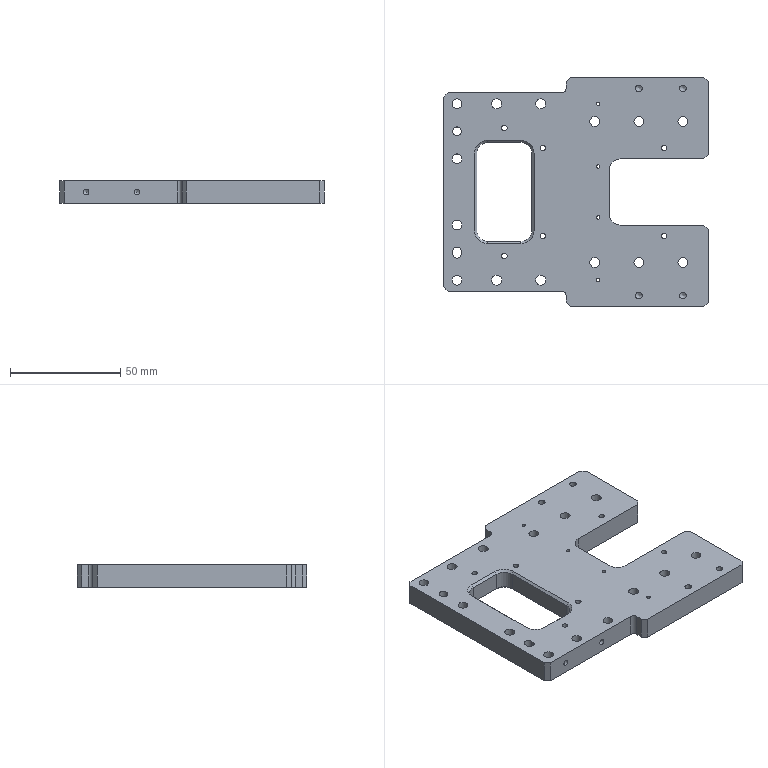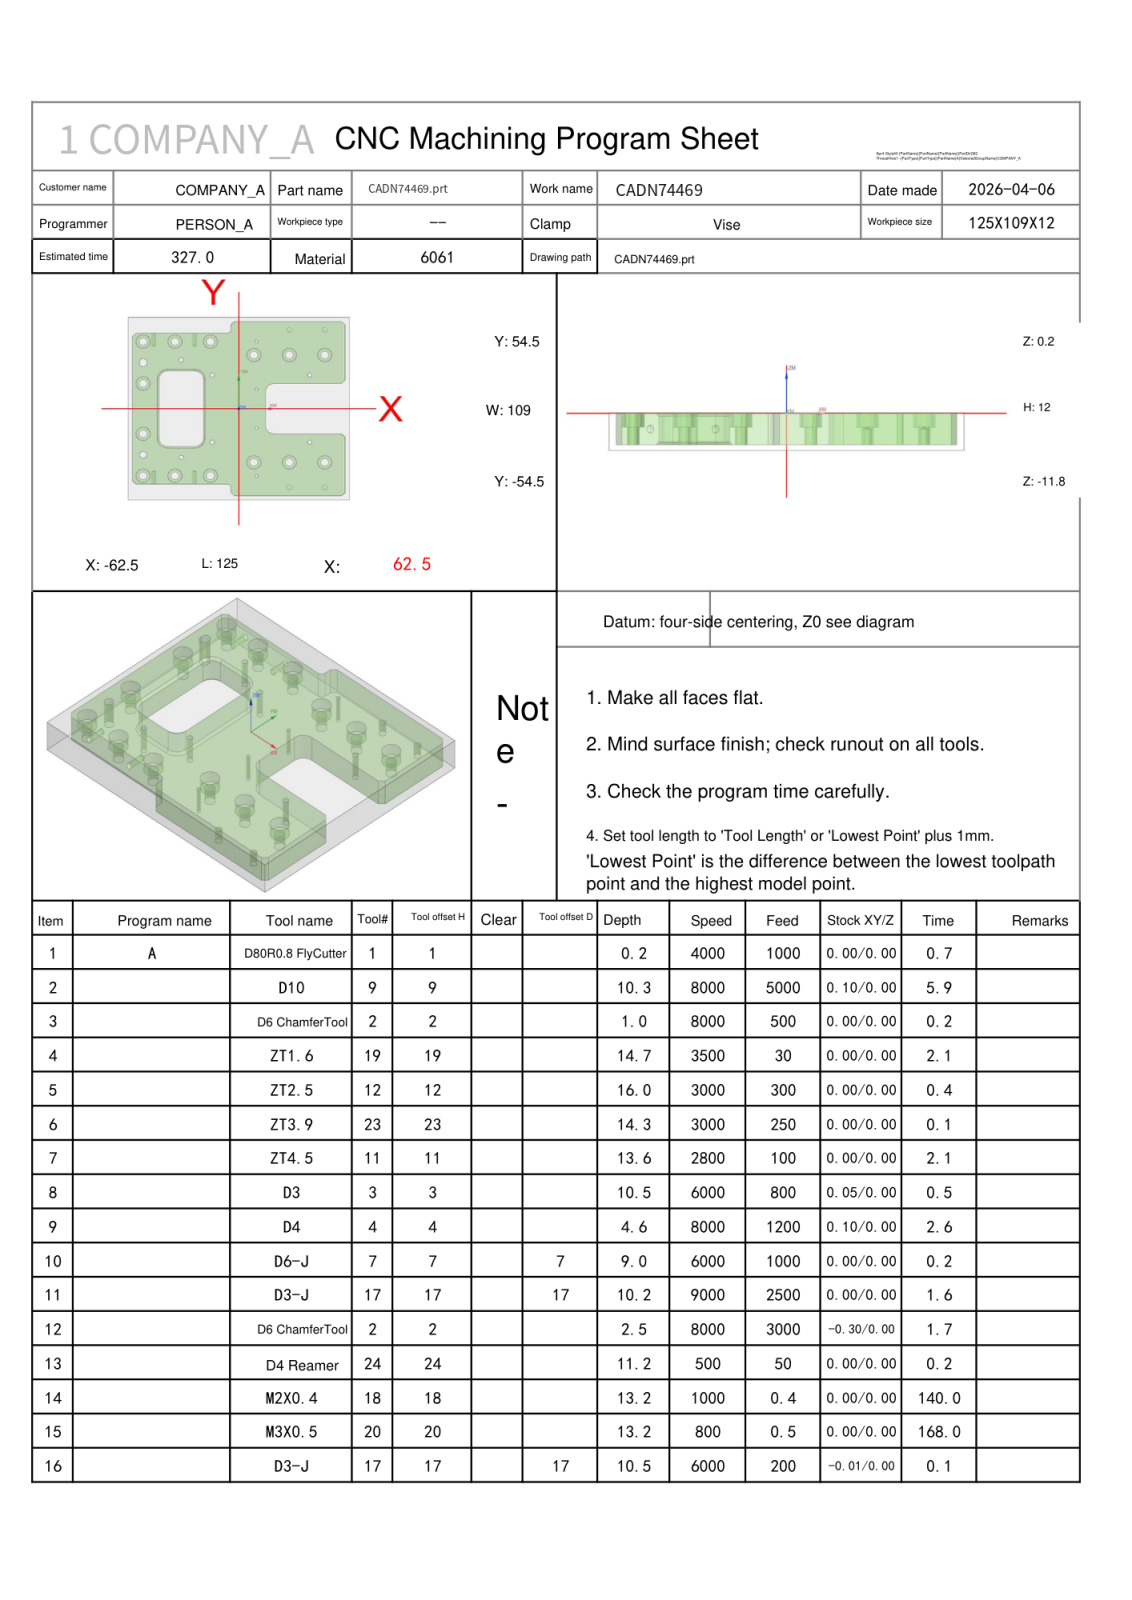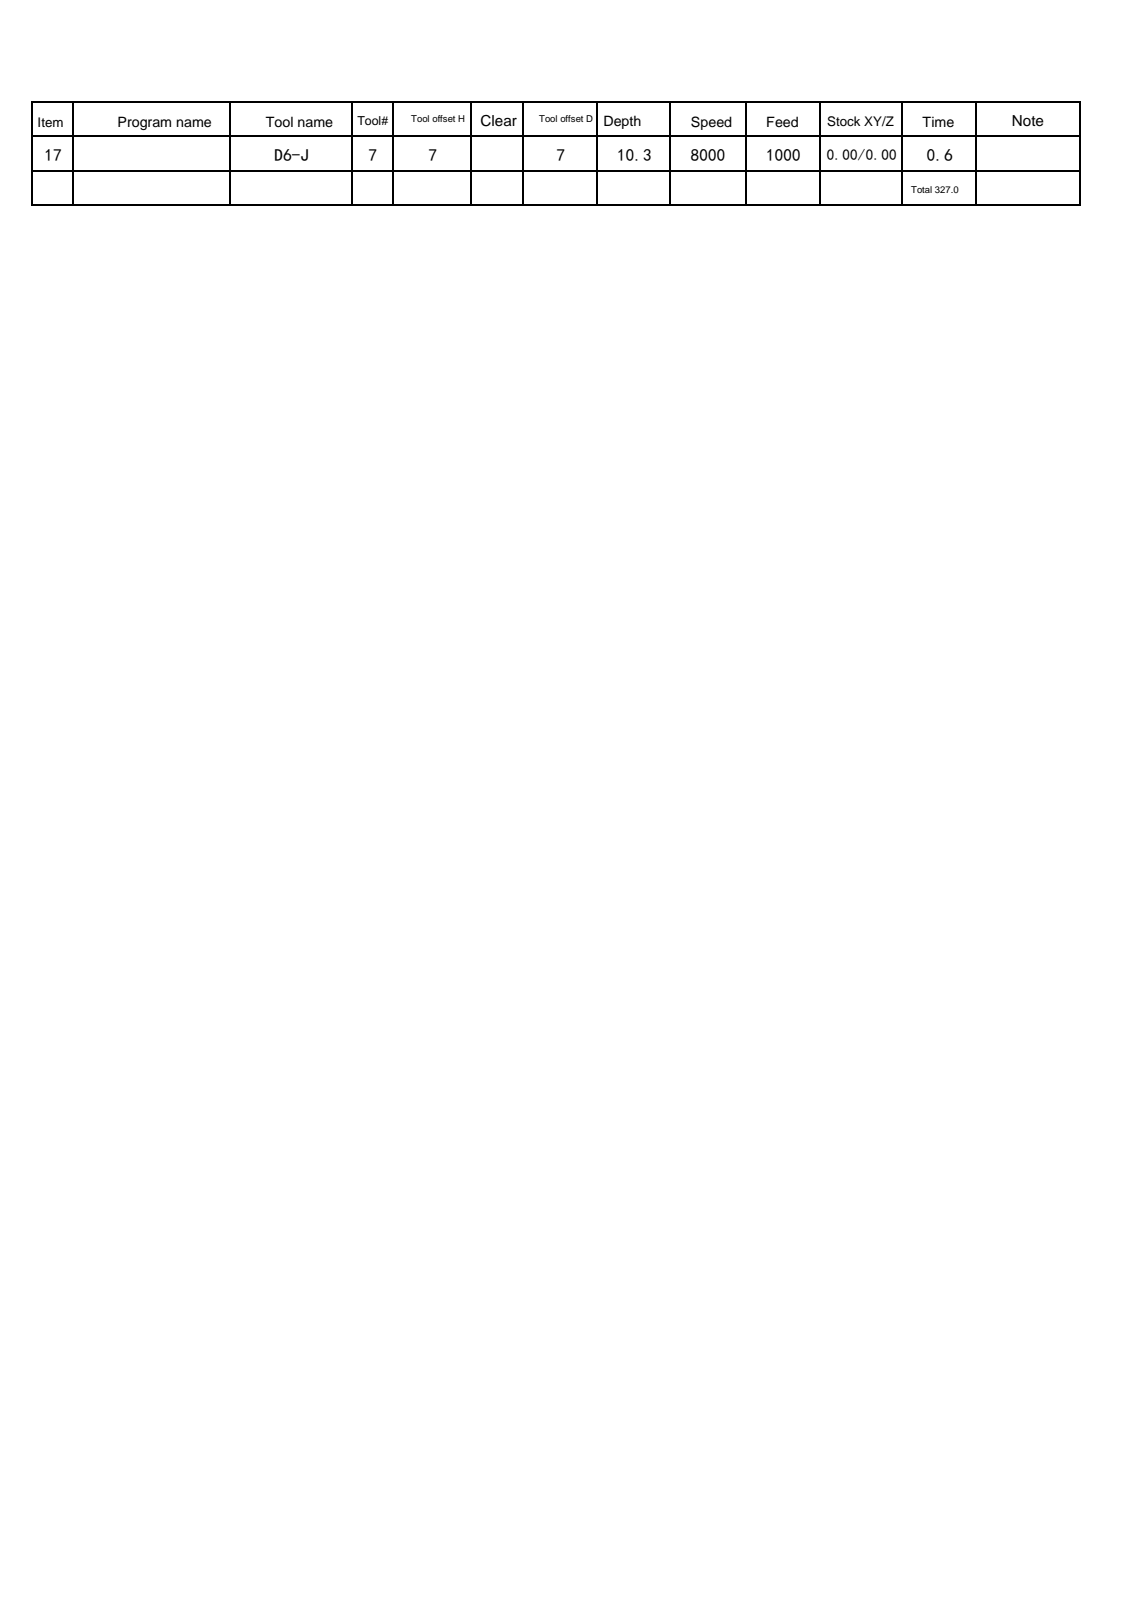NC program | NX | posted by the shop | part box 120 x 104 x 10 mm
Lines 2469 to 3517 of 6435:
N3 T02 M06
(D6 ChamferTool  D=6. R=0. H=02 ce=0.00 di=0.00)
G00 G90 G54 X48.5 Y-32. M03 S8000
G43 H02 Z20.
M08
G98 G81 X48.5 Y-32. Z-.8 R1. F500.
X40. Y-20.
X28.5 Y-32.
X10. Y-40.
X8.5 Y-32.
X10. Y-11.54
Y11.54
X40. Y20.
X48.5 Y32.
X28.5
X10. Y40.
X8.5 Y32.
X-16. Y40.
X-15. Y20.
X-32.5 Y29.
X-36. Y40.
X-54.
Y15.
Y-15.
Y-27.5
Y-40.
X-36.
X-32.5 Y-29.
X-15. Y-20.
X-16. Y-40.
X-54. Y27.
G80
G00 Z20.
G91 G28 Z0.0
M05
M09
G91 G28 Z0.0
M01
N4 T19 M06
(ZT1.6 D=1.6 DR_a=118 H=19)
G00 G90 G54 X10. Y40. M03 S3500
G43 H19 Z20.
M08
G98 G83 X10. Y40. Z-14.481 R1. F30. Q1.
Y11.54
Y-11.54
Y-40.
G80
G00 Z20.
G91 G28 Z0.0
M05
M09
G91 G28 Z0.0
M01
N5 T12 M06
(ZT2.5 D=2.5 DR_a=118 H=12)
G00 G90 G54 X40. Y20. M03 S3000
G43 H12 Z20.
M08
G98 G83 X40. Y20. Z-15.751 R1. F300. Q2.
Y-20.
X-15.
X-32.5 Y-29.
X-15. Y20.
X-32.5 Y29.
G80
G00 Z20.
G91 G28 Z0.0
M05
M09
G91 G28 Z0.0
M01
N6 T23 M06
(ZT3.9 D=3.9 DR_a=120 H=23)
G00 G90 G54 X-54. Y-27.5 M03 S3000
G43 H23 Z20.
M08
G98 G83 X-54. Y-27.5 Z-14.126 R1. F250. Q2.
Y27.
G80
G00 Z20.
G91 G28 Z0.0
M05
M09
G91 G28 Z0.0
M01
N7 T11 M06
(ZT4.5 D=4.5 DR_a=118 H=11)
G00 G90 G54 X48.5 Y-32. M03 S2800
G43 H11 Z20.
M08
G98 G83 X48.5 Y-32. Z-13.352 R1. F100. Q2.
X28.5
X8.5
X-16. Y-40.
X-36.
X-54.
Y-15.
Y15.
Y40.
X-36.
X-16.
X8.5 Y32.
X28.5
X48.5
G80
G00 Z20.
G91 G28 Z0.0
M05
M09
G91 G28 Z0.0
M01
N8 T03 M06
(D3  D=3. R=0. H=03 ce=0.05 di=0.00)
G00 G90 G54 X-54.45 Y27.5 M03 S6000
G43 H03 Z20.
M08
Z.5
G01 Y27. Z.485 F800.
G03 X-54. Y26.55 Z.463 I.45 J0.0
X-53.55 Y27. Z.441 I0.0 J.45
G01 Y28. Z.411
G03 X-54. Y28.45 Z.389 I-.45 J0.0
X-54.45 Y28. Z.367 I0.0 J-.45
G01 Y27. Z.337
G03 X-54. Y26.55 Z.315 I.45 J0.0
X-53.55 Y27. Z.293 I0.0 J.45
G01 Y28. Z.263
G03 X-54. Y28.45 Z.241 I-.45 J0.0
X-54.45 Y28. Z.219 I0.0 J-.45
G01 Y27. Z.189
G03 X-54. Y26.55 Z.167 I.45 J0.0
X-53.55 Y27. Z.145 I0.0 J.45
G01 Y28. Z.115
G03 X-54. Y28.45 Z.093 I-.45 J0.0
X-54.45 Y28. Z.071 I0.0 J-.45
G01 Y27. Z.041
G03 X-54. Y26.55 Z.019 I.45 J0.0
X-53.55 Y27. Z-.002 I0.0 J.45
G01 Y28. Z-.033
G03 X-54. Y28.45 Z-.055 I-.45 J0.0
X-54.45 Y28. Z-.076 I0.0 J-.45
G01 Y27. Z-.107
G03 X-54. Y26.55 Z-.129 I.45 J0.0
X-53.55 Y27. Z-.15 I0.0 J.45
G01 Y28. Z-.181
G03 X-54. Y28.45 Z-.203 I-.45 J0.0
X-54.45 Y28. Z-.224 I0.0 J-.45
G01 Y27. Z-.255
G03 X-54. Y26.55 Z-.277 I.45 J0.0
X-53.55 Y27. Z-.298 I0.0 J.45
G01 Y28. Z-.329
G03 X-54. Y28.45 Z-.351 I-.45 J0.0
X-54.45 Y28. Z-.372 I0.0 J-.45
G01 Y27. Z-.403
G03 X-54. Y26.55 Z-.425 I.45 J0.0
X-53.55 Y27. Z-.446 I0.0 J.45
G01 Y28. Z-.477
G03 X-54. Y28.45 Z-.499 I-.45 J0.0
X-54.45 Y28. Z-.52 I0.0 J-.45
G01 Y27. Z-.551
G03 X-54. Y26.55 Z-.573 I.45 J0.0
X-53.55 Y27. Z-.594 I0.0 J.45
G01 Y28. Z-.625
G03 X-54. Y28.45 Z-.647 I-.45 J0.0
X-54.45 Y28. Z-.668 I0.0 J-.45
G01 Y27. Z-.699
G03 X-54. Y26.55 Z-.721 I.45 J0.0
X-53.55 Y27. Z-.742 I0.0 J.45
G01 Y28. Z-.773
G03 X-54. Y28.45 Z-.795 I-.45 J0.0
X-54.45 Y28. Z-.816 I0.0 J-.45
G01 Y27. Z-.847
G03 X-54. Y26.55 Z-.868 I.45 J0.0
X-53.55 Y27. Z-.89 I0.0 J.45
G01 Y28. Z-.921
G03 X-54. Y28.45 Z-.942 I-.45 J0.0
X-54.45 Y28. Z-.964 I0.0 J-.45
G01 Y27. Z-.995
G03 X-54. Y26.55 Z-1.016 I.45 J0.0
X-53.55 Y27. Z-1.038 I0.0 J.45
G01 Y28. Z-1.069
G03 X-54. Y28.45 Z-1.09 I-.45 J0.0
X-54.45 Y28. Z-1.112 I0.0 J-.45
G01 Y27. Z-1.143
G03 X-54. Y26.55 Z-1.164 I.45 J0.0
X-53.55 Y27. Z-1.186 I0.0 J.45
G01 Y28. Z-1.217
G03 X-54. Y28.45 Z-1.238 I-.45 J0.0
X-54.45 Y28. Z-1.26 I0.0 J-.45
G01 Y27. Z-1.291
G03 X-54. Y26.55 Z-1.312 I.45 J0.0
X-53.55 Y27. Z-1.334 I0.0 J.45
G01 Y28. Z-1.365
G03 X-54. Y28.45 Z-1.386 I-.45 J0.0
X-54.45 Y28. Z-1.408 I0.0 J-.45
G01 Y27. Z-1.439
G03 X-54. Y26.55 Z-1.46 I.45 J0.0
X-53.55 Y27. Z-1.482 I0.0 J.45
G01 Y28. Z-1.513
G03 X-54. Y28.45 Z-1.534 I-.45 J0.0
X-54.45 Y28. Z-1.556 I0.0 J-.45
G01 Y27. Z-1.587
G03 X-54. Y26.55 Z-1.608 I.45 J0.0
X-53.55 Y27. Z-1.63 I0.0 J.45
G01 Y28. Z-1.661
G03 X-54. Y28.45 Z-1.682 I-.45 J0.0
X-54.45 Y28. Z-1.704 I0.0 J-.45
G01 Y27. Z-1.735
G03 X-54. Y26.55 Z-1.756 I.45 J0.0
X-53.55 Y27. Z-1.778 I0.0 J.45
G01 Y28. Z-1.808
G03 X-54. Y28.45 Z-1.83 I-.45 J0.0
X-54.45 Y28. Z-1.852 I0.0 J-.45
G01 Y27. Z-1.882
G03 X-54. Y26.55 Z-1.904 I.45 J0.0
X-53.55 Y27. Z-1.926 I0.0 J.45
G01 Y28. Z-1.956
G03 X-54. Y28.45 Z-1.978 I-.45 J0.0
X-54.45 Y28. Z-2. I0.0 J-.45
G01 Y27. Z-2.03
G03 X-54. Y26.55 Z-2.052 I.45 J0.0
X-53.55 Y27. Z-2.074 I0.0 J.45
G01 Y28. Z-2.104
G03 X-54. Y28.45 Z-2.126 I-.45 J0.0
X-54.45 Y28. Z-2.148 I0.0 J-.45
G01 Y27. Z-2.178
G03 X-54. Y26.55 Z-2.2 I.45 J0.0
X-53.55 Y27. Z-2.222 I0.0 J.45
G01 Y28. Z-2.252
G03 X-54. Y28.45 Z-2.274 I-.45 J0.0
X-54.45 Y28. Z-2.296 I0.0 J-.45
G01 Y27. Z-2.326
G03 X-54. Y26.55 Z-2.348 I.45 J0.0
X-53.55 Y27. Z-2.37 I0.0 J.45
G01 Y28. Z-2.4
G03 X-54. Y28.45 Z-2.422 I-.45 J0.0
X-54.45 Y28. Z-2.444 I0.0 J-.45
G01 Y27. Z-2.474
G03 X-54. Y26.55 Z-2.496 I.45 J0.0
X-53.55 Y27. Z-2.518 I0.0 J.45
G01 Y28. Z-2.548
G03 X-54. Y28.45 Z-2.57 I-.45 J0.0
X-54.45 Y28. Z-2.592 I0.0 J-.45
G01 Y27. Z-2.622
G03 X-54. Y26.55 Z-2.644 I.45 J0.0
X-53.55 Y27. Z-2.665 I0.0 J.45
G01 Y28. Z-2.696
G03 X-54. Y28.45 Z-2.718 I-.45 J0.0
X-54.45 Y28. Z-2.739 I0.0 J-.45
G01 Y27. Z-2.77
G03 X-54. Y26.55 Z-2.792 I.45 J0.0
X-53.55 Y27. Z-2.813 I0.0 J.45
G01 Y28. Z-2.844
G03 X-54. Y28.45 Z-2.866 I-.45 J0.0
X-54.45 Y28. Z-2.887 I0.0 J-.45
G01 Y27. Z-2.918
G03 X-54. Y26.55 Z-2.94 I.45 J0.0
X-53.55 Y27. Z-2.961 I0.0 J.45
G01 Y28. Z-2.992
G03 X-54. Y28.45 Z-3.014 I-.45 J0.0
X-54.45 Y28. Z-3.035 I0.0 J-.45
G01 Y27. Z-3.066
G03 X-54. Y26.55 Z-3.088 I.45 J0.0
X-53.55 Y27. Z-3.109 I0.0 J.45
G01 Y28. Z-3.14
G03 X-54. Y28.45 Z-3.162 I-.45 J0.0
X-54.45 Y28. Z-3.183 I0.0 J-.45
G01 Y27. Z-3.214
G03 X-54. Y26.55 Z-3.236 I.45 J0.0
X-53.55 Y27. Z-3.257 I0.0 J.45
G01 Y28. Z-3.288
G03 X-54. Y28.45 Z-3.31 I-.45 J0.0
X-54.45 Y28. Z-3.331 I0.0 J-.45
G01 Y27. Z-3.362
G03 X-54. Y26.55 Z-3.384 I.45 J0.0
X-53.55 Y27. Z-3.405 I0.0 J.45
G01 Y28. Z-3.436
G03 X-54. Y28.45 Z-3.458 I-.45 J0.0
X-54.45 Y28. Z-3.479 I0.0 J-.45
G01 Y27. Z-3.51
G03 X-54. Y26.55 Z-3.532 I.45 J0.0
X-53.55 Y27. Z-3.553 I0.0 J.45
G01 Y28. Z-3.584
G03 X-54. Y28.45 Z-3.605 I-.45 J0.0
X-54.45 Y28. Z-3.627 I0.0 J-.45
G01 Y27. Z-3.658
G03 X-54. Y26.55 Z-3.679 I.45 J0.0
X-53.55 Y27. Z-3.701 I0.0 J.45
G01 Y28. Z-3.732
G03 X-54. Y28.45 Z-3.753 I-.45 J0.0
X-54.45 Y28. Z-3.775 I0.0 J-.45
G01 Y27. Z-3.806
G03 X-54. Y26.55 Z-3.827 I.45 J0.0
X-53.55 Y27. Z-3.849 I0.0 J.45
G01 Y28. Z-3.88
G03 X-54. Y28.45 Z-3.901 I-.45 J0.0
X-54.45 Y28. Z-3.923 I0.0 J-.45
G01 Y27. Z-3.954
G03 X-54. Y26.55 Z-3.975 I.45 J0.0
X-53.55 Y27. Z-3.997 I0.0 J.45
G01 Y28. Z-4.028
G03 X-54. Y28.45 Z-4.049 I-.45 J0.0
X-54.45 Y28. Z-4.071 I0.0 J-.45
G01 Y27. Z-4.102
G03 X-54. Y26.55 Z-4.123 I.45 J0.0
X-53.55 Y27. Z-4.145 I0.0 J.45
G01 Y28. Z-4.176
G03 X-54. Y28.45 Z-4.197 I-.45 J0.0
X-54.45 Y28. Z-4.219 I0.0 J-.45
G01 Y27. Z-4.25
G03 X-54. Y26.55 Z-4.271 I.45 J0.0
X-53.55 Y27. Z-4.293 I0.0 J.45
G01 Y28. Z-4.324
G03 X-54. Y28.45 Z-4.345 I-.45 J0.0
X-54.45 Y28. Z-4.367 I0.0 J-.45
G01 Y27. Z-4.398
G03 X-54. Y26.55 Z-4.419 I.45 J0.0
X-53.55 Y27. Z-4.441 I0.0 J.45
G01 Y28. Z-4.471
G03 X-54. Y28.45 Z-4.493 I-.45 J0.0
X-54.45 Y28. Z-4.515 I0.0 J-.45
G01 Y27. Z-4.545
G03 X-54. Y26.55 Z-4.567 I.45 J0.0
X-53.55 Y27. Z-4.589 I0.0 J.45
G01 Y28. Z-4.619
G03 X-54. Y28.45 Z-4.641 I-.45 J0.0
X-54.45 Y28. Z-4.663 I0.0 J-.45
G01 Y27. Z-4.693
G03 X-54. Y26.55 Z-4.715 I.45 J0.0
X-53.55 Y27. Z-4.737 I0.0 J.45
G01 Y28. Z-4.767
G03 X-54. Y28.45 Z-4.789 I-.45 J0.0
X-54.45 Y28. Z-4.811 I0.0 J-.45
G01 Y27. Z-4.841
G03 X-54. Y26.55 Z-4.863 I.45 J0.0
X-53.55 Y27. Z-4.885 I0.0 J.45
G01 Y28. Z-4.915
G03 X-54. Y28.45 Z-4.937 I-.45 J0.0
X-54.45 Y28. Z-4.959 I0.0 J-.45
G01 Y27. Z-4.989
G03 X-54. Y26.55 Z-5.011 I.45 J0.0
X-53.55 Y27. Z-5.033 I0.0 J.45
G01 Y28. Z-5.063
G03 X-54. Y28.45 Z-5.085 I-.45 J0.0
X-54.45 Y28. Z-5.107 I0.0 J-.45
G01 Y27. Z-5.137
G03 X-54. Y26.55 Z-5.159 I.45 J0.0
X-53.55 Y27. Z-5.181 I0.0 J.45
G01 Y28. Z-5.211
G03 X-54. Y28.45 Z-5.233 I-.45 J0.0
X-54.45 Y28. Z-5.255 I0.0 J-.45
G01 Y27. Z-5.285
G03 X-54. Y26.55 Z-5.307 I.45 J0.0
X-53.55 Y27. Z-5.329 I0.0 J.45
G01 Y28. Z-5.359
G03 X-54. Y28.45 Z-5.381 I-.45 J0.0
X-54.45 Y28. Z-5.402 I0.0 J-.45
G01 Y27. Z-5.433
G03 X-54. Y26.55 Z-5.455 I.45 J0.0
X-53.55 Y27. Z-5.476 I0.0 J.45
G01 Y28. Z-5.507
G03 X-54. Y28.45 Z-5.529 I-.45 J0.0
X-54.45 Y28. Z-5.55 I0.0 J-.45
G01 Y27. Z-5.581
G03 X-54. Y26.55 Z-5.603 I.45 J0.0
X-53.55 Y27. Z-5.624 I0.0 J.45
G01 Y28. Z-5.655
G03 X-54. Y28.45 Z-5.677 I-.45 J0.0
X-54.45 Y28. Z-5.698 I0.0 J-.45
G01 Y27. Z-5.729
G03 X-54. Y26.55 Z-5.751 I.45 J0.0
X-53.55 Y27. Z-5.772 I0.0 J.45
G01 Y28. Z-5.803
G03 X-54. Y28.45 Z-5.825 I-.45 J0.0
X-54.45 Y28. Z-5.846 I0.0 J-.45
G01 Y27. Z-5.877
G03 X-54. Y26.55 Z-5.899 I.45 J0.0
X-53.55 Y27. Z-5.92 I0.0 J.45
G01 Y28. Z-5.951
G03 X-54. Y28.45 Z-5.973 I-.45 J0.0
X-54.45 Y28. Z-5.994 I0.0 J-.45
G01 Y27. Z-6.025
G03 X-54. Y26.55 Z-6.047 I.45 J0.0
X-53.55 Y27. Z-6.068 I0.0 J.45
G01 Y28. Z-6.099
G03 X-54. Y28.45 Z-6.121 I-.45 J0.0
X-54.45 Y28. Z-6.142 I0.0 J-.45
G01 Y27. Z-6.173
G03 X-54. Y26.55 Z-6.195 I.45 J0.0
X-53.55 Y27. Z-6.216 I0.0 J.45
G01 Y28. Z-6.247
G03 X-54. Y28.45 Z-6.268 I-.45 J0.0
X-54.45 Y28. Z-6.29 I0.0 J-.45
G01 Y27. Z-6.321
G03 X-54. Y26.55 Z-6.342 I.45 J0.0
X-53.55 Y27. Z-6.364 I0.0 J.45
G01 Y28. Z-6.395
G03 X-54. Y28.45 Z-6.416 I-.45 J0.0
X-54.45 Y28. Z-6.438 I0.0 J-.45
G01 Y27. Z-6.469
G03 X-54. Y26.55 Z-6.49 I.45 J0.0
X-53.55 Y27. Z-6.512 I0.0 J.45
G01 Y28. Z-6.543
G03 X-54. Y28.45 Z-6.564 I-.45 J0.0
X-54.45 Y28. Z-6.586 I0.0 J-.45
G01 Y27. Z-6.617
G03 X-54. Y26.55 Z-6.638 I.45 J0.0
X-53.55 Y27. Z-6.66 I0.0 J.45
G01 Y28. Z-6.691
G03 X-54. Y28.45 Z-6.712 I-.45 J0.0
X-54.45 Y28. Z-6.734 I0.0 J-.45
G01 Y27. Z-6.765
G03 X-54. Y26.55 Z-6.786 I.45 J0.0
X-53.55 Y27. Z-6.808 I0.0 J.45
G01 Y28. Z-6.839
G03 X-54. Y28.45 Z-6.86 I-.45 J0.0
X-54.45 Y28. Z-6.882 I0.0 J-.45
G01 Y27. Z-6.913
G03 X-54. Y26.55 Z-6.934 I.45 J0.0
X-53.55 Y27. Z-6.956 I0.0 J.45
G01 Y28. Z-6.987
G03 X-54. Y28.45 Z-7.008 I-.45 J0.0
X-54.45 Y28. Z-7.03 I0.0 J-.45
G01 Y27. Z-7.061
G03 X-54. Y26.55 Z-7.082 I.45 J0.0
X-53.55 Y27. Z-7.104 I0.0 J.45
G01 Y28. Z-7.135
G03 X-54. Y28.45 Z-7.156 I-.45 J0.0
X-54.45 Y28. Z-7.178 I0.0 J-.45
G01 Y27. Z-7.208
G03 X-54. Y26.55 Z-7.23 I.45 J0.0
X-53.55 Y27. Z-7.252 I0.0 J.45
G01 Y28. Z-7.282
G03 X-54. Y28.45 Z-7.304 I-.45 J0.0
X-54.45 Y28. Z-7.326 I0.0 J-.45
G01 Y27. Z-7.356
G03 X-54. Y26.55 Z-7.378 I.45 J0.0
X-53.55 Y27. Z-7.4 I0.0 J.45
G01 Y28. Z-7.43
G03 X-54. Y28.45 Z-7.452 I-.45 J0.0
X-54.45 Y28. Z-7.474 I0.0 J-.45
G01 Y27. Z-7.504
G03 X-54. Y26.55 Z-7.526 I.45 J0.0
X-53.55 Y27. Z-7.548 I0.0 J.45
G01 Y28. Z-7.578
G03 X-54. Y28.45 Z-7.6 I-.45 J0.0
X-54.45 Y28. Z-7.622 I0.0 J-.45
G01 Y27. Z-7.652
G03 X-54. Y26.55 Z-7.674 I.45 J0.0
X-53.55 Y27. Z-7.696 I0.0 J.45
G01 Y28. Z-7.726
G03 X-54. Y28.45 Z-7.748 I-.45 J0.0
X-54.45 Y28. Z-7.77 I0.0 J-.45
G01 Y27. Z-7.8
G03 X-54. Y26.55 Z-7.822 I.45 J0.0
X-53.55 Y27. Z-7.844 I0.0 J.45
G01 Y28. Z-7.874
G03 X-54. Y28.45 Z-7.896 I-.45 J0.0
X-54.45 Y28. Z-7.918 I0.0 J-.45
G01 Y27. Z-7.948
G03 X-54. Y26.55 Z-7.97 I.45 J0.0
X-53.55 Y27. Z-7.992 I0.0 J.45
G01 Y28. Z-8.022
G03 X-54. Y28.45 Z-8.044 I-.45 J0.0
X-54.45 Y28. Z-8.065 I0.0 J-.45
G01 Y27. Z-8.096
G03 X-54. Y26.55 Z-8.118 I.45 J0.0
X-53.55 Y27. Z-8.139 I0.0 J.45
G01 Y28. Z-8.17
G03 X-54. Y28.45 Z-8.192 I-.45 J0.0
X-54.45 Y28. Z-8.213 I0.0 J-.45
G01 Y27. Z-8.244
G03 X-54. Y26.55 Z-8.266 I.45 J0.0
X-53.55 Y27. Z-8.287 I0.0 J.45
G01 Y28. Z-8.318
G03 X-54. Y28.45 Z-8.34 I-.45 J0.0
X-54.45 Y28. Z-8.361 I0.0 J-.45
G01 Y27. Z-8.392
G03 X-54. Y26.55 Z-8.414 I.45 J0.0
X-53.55 Y27. Z-8.435 I0.0 J.45
G01 Y28. Z-8.466
G03 X-54. Y28.45 Z-8.488 I-.45 J0.0
X-54.45 Y28. Z-8.509 I0.0 J-.45
G01 Y27. Z-8.54
G03 X-54. Y26.55 Z-8.562 I.45 J0.0
X-53.55 Y27. Z-8.583 I0.0 J.45
G01 Y28. Z-8.614
G03 X-54. Y28.45 Z-8.636 I-.45 J0.0
X-54.45 Y28. Z-8.657 I0.0 J-.45
G01 Y27. Z-8.688
G03 X-54. Y26.55 Z-8.71 I.45 J0.0
X-53.55 Y27. Z-8.731 I0.0 J.45
G01 Y28. Z-8.762
G03 X-54. Y28.45 Z-8.784 I-.45 J0.0
X-54.45 Y28. Z-8.805 I0.0 J-.45
G01 Y27. Z-8.836
G03 X-54. Y26.55 Z-8.858 I.45 J0.0
X-53.55 Y27. Z-8.879 I0.0 J.45
G01 Y28. Z-8.91
G03 X-54. Y28.45 Z-8.932 I-.45 J0.0
X-54.45 Y28. Z-8.953 I0.0 J-.45
G01 Y27. Z-8.984
G03 X-54. Y26.55 Z-9.005 I.45 J0.0
X-53.55 Y27. Z-9.027 I0.0 J.45
G01 Y28. Z-9.058
G03 X-54. Y28.45 Z-9.079 I-.45 J0.0
X-54.45 Y28. Z-9.101 I0.0 J-.45
G01 Y27. Z-9.132
G03 X-54. Y26.55 Z-9.153 I.45 J0.0
X-53.55 Y27. Z-9.175 I0.0 J.45
G01 Y28. Z-9.206
G03 X-54. Y28.45 Z-9.227 I-.45 J0.0
X-54.45 Y28. Z-9.249 I0.0 J-.45
G01 Y27. Z-9.28
G03 X-54. Y26.55 Z-9.301 I.45 J0.0
X-53.55 Y27. Z-9.323 I0.0 J.45
G01 Y28. Z-9.354
G03 X-54. Y28.45 Z-9.375 I-.45 J0.0
X-54.45 Y28. Z-9.397 I0.0 J-.45
G01 Y27. Z-9.428
G03 X-54. Y26.55 Z-9.449 I.45 J0.0
X-53.55 Y27. Z-9.471 I0.0 J.45
G01 Y28. Z-9.502
G03 X-54. Y28.45 Z-9.523 I-.45 J0.0
X-54.45 Y28. Z-9.545 I0.0 J-.45
G01 Y27. Z-9.576
G03 X-54. Y26.55 Z-9.597 I.45 J0.0
X-53.55 Y27. Z-9.619 I0.0 J.45
G01 Y28. Z-9.65
G03 X-54. Y28.45 Z-9.671 I-.45 J0.0
X-54.45 Y28. Z-9.693 I0.0 J-.45
G01 Y27. Z-9.724
G03 X-54. Y26.55 Z-9.745 I.45 J0.0
X-53.55 Y27. Z-9.767 I0.0 J.45
G01 Y28. Z-9.798
G03 X-54. Y28.45 Z-9.819 I-.45 J0.0
X-54.45 Y28. Z-9.841 I0.0 J-.45
G01 Y27. Z-9.871
G03 X-54. Y26.55 Z-9.893 I.45 J0.0
X-53.55 Y27. Z-9.915 I0.0 J.45
G01 Y28. Z-9.945
G03 X-54. Y28.45 Z-9.967 I-.45 J0.0
X-54.45 Y28. Z-9.989 I0.0 J-.45
G01 Y27. Z-10.019
G03 X-54. Y26.55 Z-10.041 I.45 J0.0
X-53.55 Y27. Z-10.063 I0.0 J.45
G01 Y28. Z-10.093
G03 X-54. Y28.45 Z-10.115 I-.45 J0.0
X-54.45 Y28. Z-10.137 I0.0 J-.45
G01 Y27. Z-10.167
G03 X-54. Y26.55 Z-10.189 I.45 J0.0
X-53.55 Y27. Z-10.211 I0.0 J.45
G01 Y28. Z-10.241
G03 X-54. Y28.45 Z-10.263 I-.45 J0.0
X-54.45 Y28. Z-10.285 I0.0 J-.45
G01 Y27.5 Z-10.3
Y27.
G03 X-54. Y26.55 I.45 J0.0
X-53.55 Y27. I0.0 J.45
G01 Y28.
G03 X-54. Y28.45 I-.45 J0.0
X-54.45 Y28. I0.0 J-.45
G01 Y27.5
Y27.
Z-9.3
G00 Z20.
G91 G28 Z0.0
M05
M09
G91 G28 Z0.0
M01
N9 T04 M06
(D4  D=4. R=0. H=04 ce=0.10 di=0.00)
G00 G90 G54 X-54. Y15. M03 S8000
G43 H04 Z20.
M08
Z.5
G03 X-53.05 Y14.05 I.95 J0.0 F1200.
X-52.1 Y15. I0.0 J.95
X-52.1 Y15. Z.2 I-1.9 J0.0
X-52.1 Y15. Z-.1 I-1.9 J0.0
X-52.1 Y15. Z-.4 I-1.9 J0.0
X-52.1 Y15. Z-.7 I-1.9 J0.0
X-52.1 Y15. Z-1. I-1.9 J0.0
X-52.1 Y15. Z-1.3 I-1.9 J0.0
X-52.1 Y15. Z-1.6 I-1.9 J0.0
X-52.1 Y15. Z-1.9 I-1.9 J0.0
X-52.1 Y15. Z-2.2 I-1.9 J0.0
X-52.1 Y15. Z-2.5 I-1.9 J0.0
X-52.1 Y15. Z-2.8 I-1.9 J0.0
X-52.1 Y15. Z-3.1 I-1.9 J0.0
X-52.1 Y15. Z-3.4 I-1.9 J0.0
X-52.1 Y15. Z-3.7 I-1.9 J0.0
X-52.1 Y15. Z-4. I-1.9 J0.0
X-52.1 Y15. Z-4.3 I-1.9 J0.0
X-54.95 Y16.645 Z-4.4 I-1.9 J0.0
X-55.9 Y15. I.95 J-1.645
X-54. Y13.1 I1.9 J0.0
X-52.1 Y15. I0.0 J1.9
X-54. Y16.9 I-1.9 J0.0
X-54.95 Y16.645 I0.0 J-1.9
X-55.425 Y15.823 I.475 J-.823
X-54.475 Y14.873 I.95 J0.0
X-54. Y15. I0.0 J.95
G00 Z20.
Y40.
Z.5
G03 X-53.05 Y39.05 I.95 J0.0
X-52.1 Y40. I0.0 J.95
X-52.1 Y40. Z.2 I-1.9 J0.0
X-52.1 Y40. Z-.1 I-1.9 J0.0
X-52.1 Y40. Z-.4 I-1.9 J0.0
X-52.1 Y40. Z-.7 I-1.9 J0.0
X-52.1 Y40. Z-1. I-1.9 J0.0
X-52.1 Y40. Z-1.3 I-1.9 J0.0
X-52.1 Y40. Z-1.6 I-1.9 J0.0
X-52.1 Y40. Z-1.9 I-1.9 J0.0
X-52.1 Y40. Z-2.2 I-1.9 J0.0
X-52.1 Y40. Z-2.5 I-1.9 J0.0
X-52.1 Y40. Z-2.8 I-1.9 J0.0
X-52.1 Y40. Z-3.1 I-1.9 J0.0
X-52.1 Y40. Z-3.4 I-1.9 J0.0
X-52.1 Y40. Z-3.7 I-1.9 J0.0
X-52.1 Y40. Z-4. I-1.9 J0.0
X-52.1 Y40. Z-4.3 I-1.9 J0.0
X-54.95 Y41.645 Z-4.4 I-1.9 J0.0
X-55.9 Y40. I.95 J-1.645
X-54. Y38.1 I1.9 J0.0
X-52.1 Y40. I0.0 J1.9
X-54. Y41.9 I-1.9 J0.0
X-54.95 Y41.645 I0.0 J-1.9
X-55.425 Y40.823 I.475 J-.823
X-54.475 Y39.873 I.95 J0.0
X-54. Y40. I0.0 J.95
G00 Z20.
X-36.
Z.5
G03 X-35.05 Y39.05 I.95 J0.0
X-34.1 Y40. I0.0 J.95
X-34.1 Y40. Z.2 I-1.9 J0.0
X-34.1 Y40. Z-.1 I-1.9 J0.0
X-34.1 Y40. Z-.4 I-1.9 J0.0
X-34.1 Y40. Z-.7 I-1.9 J0.0
X-34.1 Y40. Z-1. I-1.9 J0.0
X-34.1 Y40. Z-1.3 I-1.9 J0.0
X-34.1 Y40. Z-1.6 I-1.9 J0.0
X-34.1 Y40. Z-1.9 I-1.9 J0.0
X-34.1 Y40. Z-2.2 I-1.9 J0.0
X-34.1 Y40. Z-2.5 I-1.9 J0.0
X-34.1 Y40. Z-2.8 I-1.9 J0.0
X-34.1 Y40. Z-3.1 I-1.9 J0.0
X-34.1 Y40. Z-3.4 I-1.9 J0.0
X-34.1 Y40. Z-3.7 I-1.9 J0.0
X-34.1 Y40. Z-4. I-1.9 J0.0
X-34.1 Y40. Z-4.3 I-1.9 J0.0
X-36.95 Y41.645 Z-4.4 I-1.9 J0.0
X-37.9 Y40. I.95 J-1.645
X-36. Y38.1 I1.9 J0.0
X-34.1 Y40. I0.0 J1.9
X-36. Y41.9 I-1.9 J0.0
X-36.95 Y41.645 I0.0 J-1.9
X-37.425 Y40.823 I.475 J-.823
X-36.475 Y39.873 I.95 J0.0
X-36. Y40. I0.0 J.95
G00 Z20.
X-16.
Z.5
G03 X-15.05 Y39.05 I.95 J0.0
X-14.1 Y40. I0.0 J.95
X-14.1 Y40. Z.2 I-1.9 J0.0
X-14.1 Y40. Z-.1 I-1.9 J0.0
X-14.1 Y40. Z-.4 I-1.9 J0.0
X-14.1 Y40. Z-.7 I-1.9 J0.0
X-14.1 Y40. Z-1. I-1.9 J0.0
X-14.1 Y40. Z-1.3 I-1.9 J0.0
X-14.1 Y40. Z-1.6 I-1.9 J0.0
X-14.1 Y40. Z-1.9 I-1.9 J0.0
X-14.1 Y40. Z-2.2 I-1.9 J0.0
X-14.1 Y40. Z-2.5 I-1.9 J0.0
X-14.1 Y40. Z-2.8 I-1.9 J0.0
X-14.1 Y40. Z-3.1 I-1.9 J0.0
X-14.1 Y40. Z-3.4 I-1.9 J0.0
X-14.1 Y40. Z-3.7 I-1.9 J0.0
X-14.1 Y40. Z-4. I-1.9 J0.0
X-14.1 Y40. Z-4.3 I-1.9 J0.0
X-16.95 Y41.645 Z-4.4 I-1.9 J0.0
X-17.9 Y40. I.95 J-1.645
X-16. Y38.1 I1.9 J0.0
X-14.1 Y40. I0.0 J1.9
X-16. Y41.9 I-1.9 J0.0
X-16.95 Y41.645 I0.0 J-1.9
X-17.425 Y40.823 I.475 J-.823
X-16.475 Y39.873 I.95 J0.0
X-16. Y40. I0.0 J.95
G00 Z20.
X8.5 Y32.
Z.5
G03 X9.45 Y31.05 I.95 J0.0
X10.4 Y32. I0.0 J.95
X10.4 Y32. Z.2 I-1.9 J0.0
X10.4 Y32. Z-.1 I-1.9 J0.0
X10.4 Y32. Z-.4 I-1.9 J0.0
X10.4 Y32. Z-.7 I-1.9 J0.0
X10.4 Y32. Z-1. I-1.9 J0.0
X10.4 Y32. Z-1.3 I-1.9 J0.0
X10.4 Y32. Z-1.6 I-1.9 J0.0
X10.4 Y32. Z-1.9 I-1.9 J0.0
X10.4 Y32. Z-2.2 I-1.9 J0.0
X10.4 Y32. Z-2.5 I-1.9 J0.0
X10.4 Y32. Z-2.8 I-1.9 J0.0
X10.4 Y32. Z-3.1 I-1.9 J0.0
X10.4 Y32. Z-3.4 I-1.9 J0.0
X10.4 Y32. Z-3.7 I-1.9 J0.0
X10.4 Y32. Z-4. I-1.9 J0.0
X10.4 Y32. Z-4.3 I-1.9 J0.0
X7.55 Y33.645 Z-4.4 I-1.9 J0.0
X6.6 Y32. I.95 J-1.645
X8.5 Y30.1 I1.9 J0.0
X10.4 Y32. I0.0 J1.9
X8.5 Y33.9 I-1.9 J0.0
X7.55 Y33.645 I0.0 J-1.9
X7.075 Y32.823 I.475 J-.823
X8.025 Y31.873 I.95 J0.0
X8.5 Y32. I0.0 J.95
G00 Z20.
X28.5
Z.5
G03 X29.45 Y31.05 I.95 J0.0
X30.4 Y32. I0.0 J.95
X30.4 Y32. Z.2 I-1.9 J0.0
X30.4 Y32. Z-.1 I-1.9 J0.0
X30.4 Y32. Z-.4 I-1.9 J0.0
X30.4 Y32. Z-.7 I-1.9 J0.0
X30.4 Y32. Z-1. I-1.9 J0.0
X30.4 Y32. Z-1.3 I-1.9 J0.0
X30.4 Y32. Z-1.6 I-1.9 J0.0
X30.4 Y32. Z-1.9 I-1.9 J0.0
X30.4 Y32. Z-2.2 I-1.9 J0.0
X30.4 Y32. Z-2.5 I-1.9 J0.0
X30.4 Y32. Z-2.8 I-1.9 J0.0
X30.4 Y32. Z-3.1 I-1.9 J0.0
X30.4 Y32. Z-3.4 I-1.9 J0.0
X30.4 Y32. Z-3.7 I-1.9 J0.0
X30.4 Y32. Z-4. I-1.9 J0.0
X30.4 Y32. Z-4.3 I-1.9 J0.0
X27.55 Y33.645 Z-4.4 I-1.9 J0.0
X26.6 Y32. I.95 J-1.645
X28.5 Y30.1 I1.9 J0.0
X30.4 Y32. I0.0 J1.9
X28.5 Y33.9 I-1.9 J0.0
X27.55 Y33.645 I0.0 J-1.9
X27.075 Y32.823 I.475 J-.823
X28.025 Y31.873 I.95 J0.0
X28.5 Y32. I0.0 J.95
G00 Z20.
X48.5
Z.5
G03 X49.45 Y31.05 I.95 J0.0
X50.4 Y32. I0.0 J.95
X50.4 Y32. Z.2 I-1.9 J0.0
X50.4 Y32. Z-.1 I-1.9 J0.0
X50.4 Y32. Z-.4 I-1.9 J0.0
X50.4 Y32. Z-.7 I-1.9 J0.0
X50.4 Y32. Z-1. I-1.9 J0.0
X50.4 Y32. Z-1.3 I-1.9 J0.0
X50.4 Y32. Z-1.6 I-1.9 J0.0
X50.4 Y32. Z-1.9 I-1.9 J0.0
X50.4 Y32. Z-2.2 I-1.9 J0.0
X50.4 Y32. Z-2.5 I-1.9 J0.0
X50.4 Y32. Z-2.8 I-1.9 J0.0
X50.4 Y32. Z-3.1 I-1.9 J0.0
X50.4 Y32. Z-3.4 I-1.9 J0.0
X50.4 Y32. Z-3.7 I-1.9 J0.0
X50.4 Y32. Z-4. I-1.9 J0.0
X50.4 Y32. Z-4.3 I-1.9 J0.0
X47.55 Y33.645 Z-4.4 I-1.9 J0.0
X46.6 Y32. I.95 J-1.645
X48.5 Y30.1 I1.9 J0.0
X50.4 Y32. I0.0 J1.9
X48.5 Y33.9 I-1.9 J0.0
X47.55 Y33.645 I0.0 J-1.9
X47.075 Y32.823 I.475 J-.823
X48.025 Y31.873 I.95 J0.0
X48.5 Y32. I0.0 J.95
G00 Z20.
Y-32.
Z.5
G03 X49.45 Y-32.95 I.95 J0.0
X50.4 Y-32. I0.0 J.95
X50.4 Y-32. Z.2 I-1.9 J0.0
X50.4 Y-32. Z-.1 I-1.9 J0.0
X50.4 Y-32. Z-.4 I-1.9 J0.0
X50.4 Y-32. Z-.7 I-1.9 J0.0
X50.4 Y-32. Z-1. I-1.9 J0.0
X50.4 Y-32. Z-1.3 I-1.9 J0.0
X50.4 Y-32. Z-1.6 I-1.9 J0.0
X50.4 Y-32. Z-1.9 I-1.9 J0.0
X50.4 Y-32. Z-2.2 I-1.9 J0.0
X50.4 Y-32. Z-2.5 I-1.9 J0.0
X50.4 Y-32. Z-2.8 I-1.9 J0.0
X50.4 Y-32. Z-3.1 I-1.9 J0.0
X50.4 Y-32. Z-3.4 I-1.9 J0.0
X50.4 Y-32. Z-3.7 I-1.9 J0.0
X50.4 Y-32. Z-4. I-1.9 J0.0
X50.4 Y-32. Z-4.3 I-1.9 J0.0
X47.55 Y-30.355 Z-4.4 I-1.9 J0.0
X46.6 Y-32. I.95 J-1.645
X48.5 Y-33.9 I1.9 J0.0
X50.4 Y-32. I0.0 J1.9
X48.5 Y-30.1 I-1.9 J0.0
X47.55 Y-30.355 I0.0 J-1.9
X47.075 Y-31.177 I.475 J-.823
X48.025 Y-32.127 I.95 J0.0
X48.5 Y-32. I0.0 J.95
G00 Z20.
X28.5
Z.5
G03 X29.45 Y-32.95 I.95 J0.0
X30.4 Y-32. I0.0 J.95
X30.4 Y-32. Z.2 I-1.9 J0.0
X30.4 Y-32. Z-.1 I-1.9 J0.0
X30.4 Y-32. Z-.4 I-1.9 J0.0
X30.4 Y-32. Z-.7 I-1.9 J0.0
X30.4 Y-32. Z-1. I-1.9 J0.0
X30.4 Y-32. Z-1.3 I-1.9 J0.0
X30.4 Y-32. Z-1.6 I-1.9 J0.0
X30.4 Y-32. Z-1.9 I-1.9 J0.0
X30.4 Y-32. Z-2.2 I-1.9 J0.0
X30.4 Y-32. Z-2.5 I-1.9 J0.0
X30.4 Y-32. Z-2.8 I-1.9 J0.0
X30.4 Y-32. Z-3.1 I-1.9 J0.0
X30.4 Y-32. Z-3.4 I-1.9 J0.0
X30.4 Y-32. Z-3.7 I-1.9 J0.0
X30.4 Y-32. Z-4. I-1.9 J0.0
X30.4 Y-32. Z-4.3 I-1.9 J0.0
X27.55 Y-30.355 Z-4.4 I-1.9 J0.0
X26.6 Y-32. I.95 J-1.645
X28.5 Y-33.9 I1.9 J0.0
X30.4 Y-32. I0.0 J1.9
X28.5 Y-30.1 I-1.9 J0.0
X27.55 Y-30.355 I0.0 J-1.9
X27.075 Y-31.177 I.475 J-.823
X28.025 Y-32.127 I.95 J0.0
X28.5 Y-32. I0.0 J.95
G00 Z20.
X8.5
Z.5
G03 X9.45 Y-32.95 I.95 J0.0
X10.4 Y-32. I0.0 J.95
X10.4 Y-32. Z.2 I-1.9 J0.0
X10.4 Y-32. Z-.1 I-1.9 J0.0
X10.4 Y-32. Z-.4 I-1.9 J0.0
X10.4 Y-32. Z-.7 I-1.9 J0.0
X10.4 Y-32. Z-1. I-1.9 J0.0
X10.4 Y-32. Z-1.3 I-1.9 J0.0
X10.4 Y-32. Z-1.6 I-1.9 J0.0
X10.4 Y-32. Z-1.9 I-1.9 J0.0
X10.4 Y-32. Z-2.2 I-1.9 J0.0
X10.4 Y-32. Z-2.5 I-1.9 J0.0
X10.4 Y-32. Z-2.8 I-1.9 J0.0
X10.4 Y-32. Z-3.1 I-1.9 J0.0
X10.4 Y-32. Z-3.4 I-1.9 J0.0
X10.4 Y-32. Z-3.7 I-1.9 J0.0
X10.4 Y-32. Z-4. I-1.9 J0.0
X10.4 Y-32. Z-4.3 I-1.9 J0.0
X7.55 Y-30.355 Z-4.4 I-1.9 J0.0
X6.6 Y-32. I.95 J-1.645
X8.5 Y-33.9 I1.9 J0.0
X10.4 Y-32. I0.0 J1.9
X8.5 Y-30.1 I-1.9 J0.0
X7.55 Y-30.355 I0.0 J-1.9
X7.075 Y-31.177 I.475 J-.823
X8.025 Y-32.127 I.95 J0.0
X8.5 Y-32. I0.0 J.95
G00 Z20.
X-16. Y-40.
Z.5
G03 X-15.05 Y-40.95 I.95 J0.0
X-14.1 Y-40. I0.0 J.95
X-14.1 Y-40. Z.2 I-1.9 J0.0
X-14.1 Y-40. Z-.1 I-1.9 J0.0
X-14.1 Y-40. Z-.4 I-1.9 J0.0
X-14.1 Y-40. Z-.7 I-1.9 J0.0
X-14.1 Y-40. Z-1. I-1.9 J0.0
X-14.1 Y-40. Z-1.3 I-1.9 J0.0
X-14.1 Y-40. Z-1.6 I-1.9 J0.0
X-14.1 Y-40. Z-1.9 I-1.9 J0.0
X-14.1 Y-40. Z-2.2 I-1.9 J0.0
X-14.1 Y-40. Z-2.5 I-1.9 J0.0
X-14.1 Y-40. Z-2.8 I-1.9 J0.0
X-14.1 Y-40. Z-3.1 I-1.9 J0.0
X-14.1 Y-40. Z-3.4 I-1.9 J0.0
X-14.1 Y-40. Z-3.7 I-1.9 J0.0
X-14.1 Y-40. Z-4. I-1.9 J0.0
X-14.1 Y-40. Z-4.3 I-1.9 J0.0
X-16.95 Y-38.355 Z-4.4 I-1.9 J0.0
X-17.9 Y-40. I.95 J-1.645
X-16. Y-41.9 I1.9 J0.0
X-14.1 Y-40. I0.0 J1.9
X-16. Y-38.1 I-1.9 J0.0
X-16.95 Y-38.355 I0.0 J-1.9
X-17.425 Y-39.177 I.475 J-.823
X-16.475 Y-40.127 I.95 J0.0
X-16. Y-40. I0.0 J.95
G00 Z20.
X-36.
Z.5
G03 X-35.05 Y-40.95 I.95 J0.0
X-34.1 Y-40. I0.0 J.95
X-34.1 Y-40. Z.2 I-1.9 J0.0
X-34.1 Y-40. Z-.1 I-1.9 J0.0
X-34.1 Y-40. Z-.4 I-1.9 J0.0
X-34.1 Y-40. Z-.7 I-1.9 J0.0
X-34.1 Y-40. Z-1. I-1.9 J0.0
X-34.1 Y-40. Z-1.3 I-1.9 J0.0
X-34.1 Y-40. Z-1.6 I-1.9 J0.0
X-34.1 Y-40. Z-1.9 I-1.9 J0.0
X-34.1 Y-40. Z-2.2 I-1.9 J0.0
X-34.1 Y-40. Z-2.5 I-1.9 J0.0
X-34.1 Y-40. Z-2.8 I-1.9 J0.0
X-34.1 Y-40. Z-3.1 I-1.9 J0.0
X-34.1 Y-40. Z-3.4 I-1.9 J0.0
X-34.1 Y-40. Z-3.7 I-1.9 J0.0
X-34.1 Y-40. Z-4. I-1.9 J0.0
X-34.1 Y-40. Z-4.3 I-1.9 J0.0
X-36.95 Y-38.355 Z-4.4 I-1.9 J0.0
X-37.9 Y-40. I.95 J-1.645
X-36. Y-41.9 I1.9 J0.0
X-34.1 Y-40. I0.0 J1.9
X-36. Y-38.1 I-1.9 J0.0
X-36.95 Y-38.355 I0.0 J-1.9
X-37.425 Y-39.177 I.475 J-.823
X-36.475 Y-40.127 I.95 J0.0
X-36. Y-40. I0.0 J.95
G00 Z20.
X-54.
Z.5
G03 X-53.05 Y-40.95 I.95 J0.0
X-52.1 Y-40. I0.0 J.95
X-52.1 Y-40. Z.2 I-1.9 J0.0
X-52.1 Y-40. Z-.1 I-1.9 J0.0
X-52.1 Y-40. Z-.4 I-1.9 J0.0
X-52.1 Y-40. Z-.7 I-1.9 J0.0
X-52.1 Y-40. Z-1. I-1.9 J0.0
X-52.1 Y-40. Z-1.3 I-1.9 J0.0
X-52.1 Y-40. Z-1.6 I-1.9 J0.0
X-52.1 Y-40. Z-1.9 I-1.9 J0.0
X-52.1 Y-40. Z-2.2 I-1.9 J0.0
X-52.1 Y-40. Z-2.5 I-1.9 J0.0
X-52.1 Y-40. Z-2.8 I-1.9 J0.0
X-52.1 Y-40. Z-3.1 I-1.9 J0.0
X-52.1 Y-40. Z-3.4 I-1.9 J0.0
X-52.1 Y-40. Z-3.7 I-1.9 J0.0
X-52.1 Y-40. Z-4. I-1.9 J0.0
X-52.1 Y-40. Z-4.3 I-1.9 J0.0
X-54.95 Y-38.355 Z-4.4 I-1.9 J0.0
X-55.9 Y-40. I.95 J-1.645
X-54. Y-41.9 I1.9 J0.0
X-52.1 Y-40. I0.0 J1.9
X-54. Y-38.1 I-1.9 J0.0
X-54.95 Y-38.355 I0.0 J-1.9
X-55.425 Y-39.177 I.475 J-.823
X-54.475 Y-40.127 I.95 J0.0
X-54. Y-40. I0.0 J.95
G00 Z20.
Y-15.
Z.5
G03 X-53.05 Y-15.95 I.95 J0.0
X-52.1 Y-15. I0.0 J.95
X-52.1 Y-15. Z.2 I-1.9 J0.0
X-52.1 Y-15. Z-.1 I-1.9 J0.0
X-52.1 Y-15. Z-.4 I-1.9 J0.0
X-52.1 Y-15. Z-.7 I-1.9 J0.0
X-52.1 Y-15. Z-1. I-1.9 J0.0
X-52.1 Y-15. Z-1.3 I-1.9 J0.0
X-52.1 Y-15. Z-1.6 I-1.9 J0.0
X-52.1 Y-15. Z-1.9 I-1.9 J0.0
X-52.1 Y-15. Z-2.2 I-1.9 J0.0
X-52.1 Y-15. Z-2.5 I-1.9 J0.0
X-52.1 Y-15. Z-2.8 I-1.9 J0.0
X-52.1 Y-15. Z-3.1 I-1.9 J0.0
X-52.1 Y-15. Z-3.4 I-1.9 J0.0
X-52.1 Y-15. Z-3.7 I-1.9 J0.0
X-52.1 Y-15. Z-4. I-1.9 J0.0
X-52.1 Y-15. Z-4.3 I-1.9 J0.0
X-54.95 Y-13.355 Z-4.4 I-1.9 J0.0
X-55.9 Y-15. I.95 J-1.645
X-54. Y-16.9 I1.9 J0.0
X-52.1 Y-15. I0.0 J1.9
X-54. Y-13.1 I-1.9 J0.0
X-54.95 Y-13.355 I0.0 J-1.9
X-55.425 Y-14.177 I.475 J-.823
X-54.475 Y-15.127 I.95 J0.0
X-54. Y-15. I0.0 J.95
G00 Z20.
G91 G28 Z0.0
M05
M09
G91 G28 Z0.0
M01
N10 T07 M06
(D6-J  D=6. R=0. H=07 ce=0.00 di=0.00)
G00 G90 G54 X-39.8 Y18.5 M03 S6000
G43 H07 Z20.
M08
Z-8.
G01 Z-8.5 F1000.
G41 D07
X-41.
G03 X-42. Y17.5 I0.0 J-1.
G01 Y-17.5
G03 X-40. Y-19.5 I2. J0.0
G01 X-25.
G03 X-23. Y-17.5 I0.0 J2.
G01 Y17.5
G03 X-25. Y19.5 I-2. J0.0
G01 X-40.
G03 X-42. Y17.5 I0.0 J-2.
G01 Y17.
G03 X-41. Y16. I1. J0.0
G01 G40 X-40.8
Z-8.
G00 Z20.
G00 G90 X-39.9 Y18.5 M03 S6000
Z20.
Z-8.3
G01 Z-8.8 F1000.
G41 D07
X-41.
G03 X-42. Y17.5 I0.0 J-1.
G01 Y-17.5
G03 X-40. Y-19.5 I2. J0.0
G01 X-25.
G03 X-23. Y-17.5 I0.0 J2.
G01 Y17.5
G03 X-25. Y19.5 I-2. J0.0
G01 X-40.
G03 X-42. Y17.5 I0.0 J-2.
G01 Y17.
G03 X-41. Y16. I1. J0.0
G01 G40 X-40.9
Z-8.3
G00 Z20.
G91 G28 Z0.0
M05
M09
G91 G28 Z0.0
M01